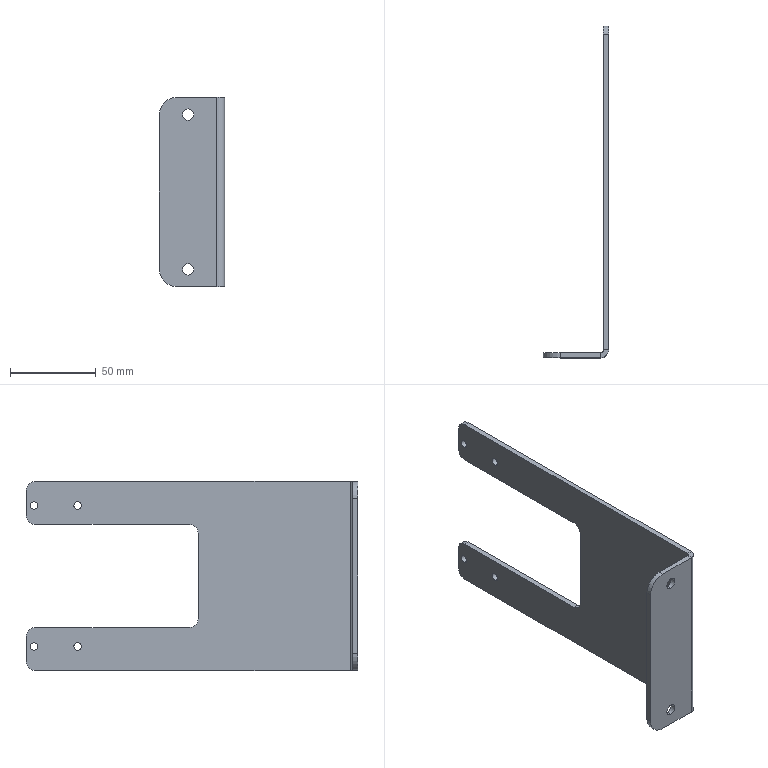Part | STEP file | 001-010-Waste through-beam photoelectric mounting plate | 1 solid | 38 faces | box 38 x 193 x 110 mm | volume 56258 mm3 | cylinder 22 | plane 16 | commonest cylinder face diameters 4.5 x8 10 x6 6.6 x4 20 x2 3 x1 9 x1